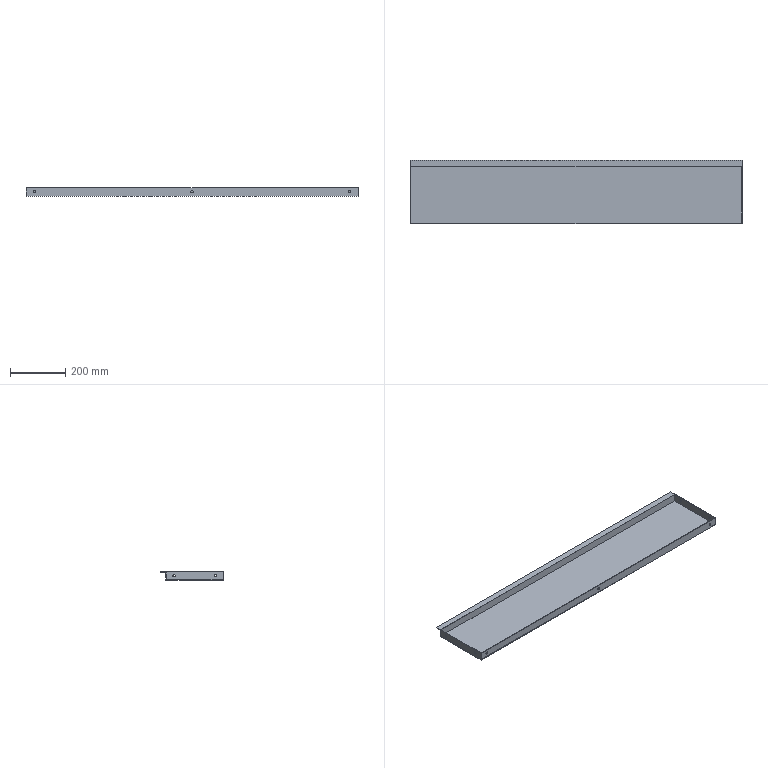Part | SolidWorks | features ICE 3, Extrusion 1, Shell 1 | 1 solid | 27 faces | box 1204 x 230 x 30 mm | volume 710869 mm3 | cylinder 14 | plane 13 | commonest cylinder face diameters 9 x14
STEP:
#1=CARTESIAN_POINT('',(602.,0.,11.5));
#2=VERTEX_POINT('',#1);
#3=CARTESIAN_POINT('',(602.,0.,20.5));
#4=VERTEX_POINT('',#3);
#5=CARTESIAN_POINT('',(602.,0.,16.));
#6=DIRECTION('',(0.,1.,0.));
#7=DIRECTION('',(0.,0.,1.));
#8=AXIS2_PLACEMENT_3D('',#5,#6,#7);
#9=CIRCLE('',#8,4.5);
#10=EDGE_CURVE('',#2,#4,#9,.T.);
#11=ORIENTED_EDGE('',*,*,#10,.F.);
#12=CARTESIAN_POINT('',(602.,2.,11.5));
#13=VERTEX_POINT('',#12);
#14=CARTESIAN_POINT('',(602.,-114.,11.5));
#15=DIRECTION('',(0.,1.,0.));
#16=VECTOR('',#15,1000.);
#17=LINE('',#14,#16);
#18=EDGE_CURVE('',#2,#13,#17,.T.);
#19=ORIENTED_EDGE('',*,*,#18,.T.);
#20=CARTESIAN_POINT('',(602.,2.,20.5));
#21=VERTEX_POINT('',#20);
#22=CARTESIAN_POINT('',(602.,2.,16.));
#23=DIRECTION('',(0.,1.,0.));
#24=DIRECTION('',(0.,0.,1.));
#25=AXIS2_PLACEMENT_3D('',#22,#23,#24);
#26=CIRCLE('',#25,4.5);
#27=EDGE_CURVE('',#13,#21,#26,.T.);
#28=ORIENTED_EDGE('',*,*,#27,.T.);
#29=CARTESIAN_POINT('',(602.,-114.,20.5));
#30=DIRECTION('',(0.,1.,0.));
#31=VECTOR('',#30,1000.);
#32=LINE('',#29,#31);
#33=EDGE_CURVE('',#4,#21,#32,.T.);
#34=ORIENTED_EDGE('',*,*,#33,.F.);
#35=EDGE_LOOP('',(#11,#19,#28,#34));
#36=FACE_OUTER_BOUND('',#35,.T.);
#37=CARTESIAN_POINT('',(602.,-114.,16.));
#38=DIRECTION('',(0.,1.,0.));
#39=DIRECTION('',(0.,0.,1.));
#40=AXIS2_PLACEMENT_3D('',#37,#38,#39);
#41=CYLINDRICAL_SURFACE('',#40,4.5);
#42=ADVANCED_FACE('',(#36),#41,.F.);
#43=CARTESIAN_POINT('',(1174.,0.,11.5));
#44=VERTEX_POINT('',#43);
#45=CARTESIAN_POINT('',(1174.,0.,20.5));
#46=VERTEX_POINT('',#45);
#47=CARTESIAN_POINT('',(1174.,0.,16.));
#48=DIRECTION('',(0.,1.,0.));
#49=DIRECTION('',(0.,0.,1.));
#50=AXIS2_PLACEMENT_3D('',#47,#48,#49);
#51=CIRCLE('',#50,4.5);
#52=EDGE_CURVE('',#44,#46,#51,.T.);
#53=ORIENTED_EDGE('',*,*,#52,.F.);
#54=CARTESIAN_POINT('',(1174.,2.,11.5));
#55=VERTEX_POINT('',#54);
#56=CARTESIAN_POINT('',(1174.,-114.,11.5));
#57=DIRECTION('',(0.,1.,0.));
#58=VECTOR('',#57,1000.);
#59=LINE('',#56,#58);
#60=EDGE_CURVE('',#44,#55,#59,.T.);
#61=ORIENTED_EDGE('',*,*,#60,.T.);
#62=CARTESIAN_POINT('',(1174.,2.,20.5));
#63=VERTEX_POINT('',#62);
#64=CARTESIAN_POINT('',(1174.,2.,16.));
#65=DIRECTION('',(0.,1.,0.));
#66=DIRECTION('',(0.,0.,1.));
#67=AXIS2_PLACEMENT_3D('',#64,#65,#66);
#68=CIRCLE('',#67,4.5);
#69=EDGE_CURVE('',#55,#63,#68,.T.);
#70=ORIENTED_EDGE('',*,*,#69,.T.);
#71=CARTESIAN_POINT('',(1174.,-114.,20.5));
#72=DIRECTION('',(0.,1.,0.));
#73=VECTOR('',#72,1000.);
#74=LINE('',#71,#73);
#75=EDGE_CURVE('',#46,#63,#74,.T.);
#76=ORIENTED_EDGE('',*,*,#75,.F.);
#77=EDGE_LOOP('',(#53,#61,#70,#76));
#78=FACE_OUTER_BOUND('',#77,.T.);
#79=CARTESIAN_POINT('',(1174.,-114.,16.));
#80=DIRECTION('',(0.,1.,0.));
#81=DIRECTION('',(0.,0.,1.));
#82=AXIS2_PLACEMENT_3D('',#79,#80,#81);
#83=CYLINDRICAL_SURFACE('',#82,4.5);
#84=ADVANCED_FACE('',(#78),#83,.F.);
#85=CARTESIAN_POINT('',(30.,0.,11.5));
#86=VERTEX_POINT('',#85);
#87=CARTESIAN_POINT('',(30.,0.,20.5));
#88=VERTEX_POINT('',#87);
#89=CARTESIAN_POINT('',(30.,0.,16.));
#90=DIRECTION('',(0.,1.,0.));
#91=DIRECTION('',(0.,0.,1.));
#92=AXIS2_PLACEMENT_3D('',#89,#90,#91);
#93=CIRCLE('',#92,4.5);
#94=EDGE_CURVE('',#86,#88,#93,.T.);
#95=ORIENTED_EDGE('',*,*,#94,.F.);
#96=CARTESIAN_POINT('',(30.,2.,11.5));
#97=VERTEX_POINT('',#96);
#98=CARTESIAN_POINT('',(30.,-114.,11.5));
#99=DIRECTION('',(0.,1.,0.));
#100=VECTOR('',#99,1000.);
#101=LINE('',#98,#100);
#102=EDGE_CURVE('',#86,#97,#101,.T.);
#103=ORIENTED_EDGE('',*,*,#102,.T.);
#104=CARTESIAN_POINT('',(30.,2.,20.5));
#105=VERTEX_POINT('',#104);
#106=CARTESIAN_POINT('',(30.,2.,16.));
#107=DIRECTION('',(0.,1.,0.));
#108=DIRECTION('',(0.,0.,1.));
#109=AXIS2_PLACEMENT_3D('',#106,#107,#108);
#110=CIRCLE('',#109,4.5);
#111=EDGE_CURVE('',#97,#105,#110,.T.);
#112=ORIENTED_EDGE('',*,*,#111,.T.);
#113=CARTESIAN_POINT('',(30.,-114.,20.5));
#114=DIRECTION('',(0.,1.,0.));
#115=VECTOR('',#114,1000.);
#116=LINE('',#113,#115);
#117=EDGE_CURVE('',#88,#105,#116,.T.);
#118=ORIENTED_EDGE('',*,*,#117,.F.);
#119=EDGE_LOOP('',(#95,#103,#112,#118));
#120=FACE_OUTER_BOUND('',#119,.T.);
#121=CARTESIAN_POINT('',(30.,-114.,16.));
#122=DIRECTION('',(0.,1.,0.));
#123=DIRECTION('',(0.,0.,1.));
#124=AXIS2_PLACEMENT_3D('',#121,#122,#123);
#125=CYLINDRICAL_SURFACE('',#124,4.5);
#126=ADVANCED_FACE('',(#120),#125,.F.);
#127=CARTESIAN_POINT('',(2.,30.,11.5));
#128=VERTEX_POINT('',#127);
#129=CARTESIAN_POINT('',(2.,30.,20.5));
#130=VERTEX_POINT('',#129);
#131=CARTESIAN_POINT('',(2.,30.,16.));
#132=DIRECTION('',(-1.,0.,0.));
#133=DIRECTION('',(0.,0.,-1.));
#134=AXIS2_PLACEMENT_3D('',#131,#132,#133);
#135=CIRCLE('',#134,4.5);
#136=EDGE_CURVE('',#128,#130,#135,.T.);
#137=ORIENTED_EDGE('',*,*,#136,.F.);
#138=CARTESIAN_POINT('',(0.,30.,11.5));
#139=VERTEX_POINT('',#138);
#140=CARTESIAN_POINT('',(1479.,30.,11.5));
#141=DIRECTION('',(-1.,0.,0.));
#142=VECTOR('',#141,1000.);
#143=LINE('',#140,#142);
#144=EDGE_CURVE('',#128,#139,#143,.T.);
#145=ORIENTED_EDGE('',*,*,#144,.T.);
#146=CARTESIAN_POINT('',(0.,30.,20.5));
#147=VERTEX_POINT('',#146);
#148=CARTESIAN_POINT('',(0.,30.,16.));
#149=DIRECTION('',(-1.,0.,0.));
#150=DIRECTION('',(0.,0.,-1.));
#151=AXIS2_PLACEMENT_3D('',#148,#149,#150);
#152=CIRCLE('',#151,4.5);
#153=EDGE_CURVE('',#139,#147,#152,.T.);
#154=ORIENTED_EDGE('',*,*,#153,.T.);
#155=CARTESIAN_POINT('',(1479.,30.,20.5));
#156=DIRECTION('',(-1.,0.,0.));
#157=VECTOR('',#156,1000.);
#158=LINE('',#155,#157);
#159=EDGE_CURVE('',#130,#147,#158,.T.);
#160=ORIENTED_EDGE('',*,*,#159,.F.);
#161=EDGE_LOOP('',(#137,#145,#154,#160));
#162=FACE_OUTER_BOUND('',#161,.T.);
#163=CARTESIAN_POINT('',(1479.,30.,16.));
#164=DIRECTION('',(-1.,0.,0.));
#165=DIRECTION('',(0.,0.,1.));
#166=AXIS2_PLACEMENT_3D('',#163,#164,#165);
#167=CYLINDRICAL_SURFACE('',#166,4.5);
#168=ADVANCED_FACE('',(#162),#167,.F.);
#169=CARTESIAN_POINT('',(1204.,30.,20.5));
#170=VERTEX_POINT('',#169);
#171=CARTESIAN_POINT('',(1204.,30.,11.5));
#172=VERTEX_POINT('',#171);
#173=CARTESIAN_POINT('',(1204.,30.,16.));
#174=DIRECTION('',(1.,0.,0.));
#175=DIRECTION('',(0.,0.,1.));
#176=AXIS2_PLACEMENT_3D('',#173,#174,#175);
#177=CIRCLE('',#176,4.5);
#178=EDGE_CURVE('',#170,#172,#177,.T.);
#179=ORIENTED_EDGE('',*,*,#178,.T.);
#180=CARTESIAN_POINT('',(1202.,30.,11.5));
#181=VERTEX_POINT('',#180);
#182=CARTESIAN_POINT('',(1479.,30.,11.5));
#183=DIRECTION('',(-1.,0.,0.));
#184=VECTOR('',#183,1000.);
#185=LINE('',#182,#184);
#186=EDGE_CURVE('',#172,#181,#185,.T.);
#187=ORIENTED_EDGE('',*,*,#186,.T.);
#188=CARTESIAN_POINT('',(1202.,30.,20.5));
#189=VERTEX_POINT('',#188);
#190=CARTESIAN_POINT('',(1202.,30.,16.));
#191=DIRECTION('',(1.,0.,0.));
#192=DIRECTION('',(0.,0.,1.));
#193=AXIS2_PLACEMENT_3D('',#190,#191,#192);
#194=CIRCLE('',#193,4.5);
#195=EDGE_CURVE('',#189,#181,#194,.T.);
#196=ORIENTED_EDGE('',*,*,#195,.F.);
#197=CARTESIAN_POINT('',(1479.,30.,20.5));
#198=DIRECTION('',(-1.,0.,0.));
#199=VECTOR('',#198,1000.);
#200=LINE('',#197,#199);
#201=EDGE_CURVE('',#170,#189,#200,.T.);
#202=ORIENTED_EDGE('',*,*,#201,.F.);
#203=EDGE_LOOP('',(#179,#187,#196,#202));
#204=FACE_OUTER_BOUND('',#203,.T.);
#205=CARTESIAN_POINT('',(1479.,30.,16.));
#206=DIRECTION('',(-1.,0.,0.));
#207=DIRECTION('',(0.,0.,1.));
#208=AXIS2_PLACEMENT_3D('',#205,#206,#207);
#209=CYLINDRICAL_SURFACE('',#208,4.5);
#210=ADVANCED_FACE('',(#204),#209,.F.);
#211=CARTESIAN_POINT('',(2.,180.,11.5));
#212=VERTEX_POINT('',#211);
#213=CARTESIAN_POINT('',(2.,180.,20.5));
#214=VERTEX_POINT('',#213);
#215=CARTESIAN_POINT('',(2.,180.,16.));
#216=DIRECTION('',(-1.,0.,0.));
#217=DIRECTION('',(0.,0.,-1.));
#218=AXIS2_PLACEMENT_3D('',#215,#216,#217);
#219=CIRCLE('',#218,4.5);
#220=EDGE_CURVE('',#212,#214,#219,.T.);
#221=ORIENTED_EDGE('',*,*,#220,.F.);
#222=CARTESIAN_POINT('',(0.,180.,11.5));
#223=VERTEX_POINT('',#222);
#224=CARTESIAN_POINT('',(1479.,180.,11.5));
#225=DIRECTION('',(-1.,0.,0.));
#226=VECTOR('',#225,1000.);
#227=LINE('',#224,#226);
#228=EDGE_CURVE('',#212,#223,#227,.T.);
#229=ORIENTED_EDGE('',*,*,#228,.T.);
#230=CARTESIAN_POINT('',(0.,180.,20.5));
#231=VERTEX_POINT('',#230);
#232=CARTESIAN_POINT('',(0.,180.,16.));
#233=DIRECTION('',(-1.,0.,0.));
#234=DIRECTION('',(0.,0.,-1.));
#235=AXIS2_PLACEMENT_3D('',#232,#233,#234);
#236=CIRCLE('',#235,4.5);
#237=EDGE_CURVE('',#223,#231,#236,.T.);
#238=ORIENTED_EDGE('',*,*,#237,.T.);
#239=CARTESIAN_POINT('',(1479.,180.,20.5));
#240=DIRECTION('',(-1.,0.,0.));
#241=VECTOR('',#240,1000.);
#242=LINE('',#239,#241);
#243=EDGE_CURVE('',#214,#231,#242,.T.);
#244=ORIENTED_EDGE('',*,*,#243,.F.);
#245=EDGE_LOOP('',(#221,#229,#238,#244));
#246=FACE_OUTER_BOUND('',#245,.T.);
#247=CARTESIAN_POINT('',(1479.,180.,16.));
#248=DIRECTION('',(-1.,0.,0.));
#249=DIRECTION('',(0.,0.,1.));
#250=AXIS2_PLACEMENT_3D('',#247,#248,#249);
#251=CYLINDRICAL_SURFACE('',#250,4.5);
#252=ADVANCED_FACE('',(#246),#251,.F.);
#253=CARTESIAN_POINT('',(1204.,180.,20.5));
#254=VERTEX_POINT('',#253);
#255=CARTESIAN_POINT('',(1204.,180.,11.5));
#256=VERTEX_POINT('',#255);
#257=CARTESIAN_POINT('',(1204.,180.,16.));
#258=DIRECTION('',(1.,0.,0.));
#259=DIRECTION('',(0.,0.,1.));
#260=AXIS2_PLACEMENT_3D('',#257,#258,#259);
#261=CIRCLE('',#260,4.5);
#262=EDGE_CURVE('',#254,#256,#261,.T.);
#263=ORIENTED_EDGE('',*,*,#262,.T.);
#264=CARTESIAN_POINT('',(1202.,180.,11.5));
#265=VERTEX_POINT('',#264);
#266=CARTESIAN_POINT('',(1479.,180.,11.5));
#267=DIRECTION('',(-1.,0.,0.));
#268=VECTOR('',#267,1000.);
#269=LINE('',#266,#268);
#270=EDGE_CURVE('',#256,#265,#269,.T.);
#271=ORIENTED_EDGE('',*,*,#270,.T.);
#272=CARTESIAN_POINT('',(1202.,180.,20.5));
#273=VERTEX_POINT('',#272);
#274=CARTESIAN_POINT('',(1202.,180.,16.));
#275=DIRECTION('',(1.,0.,0.));
#276=DIRECTION('',(0.,0.,1.));
#277=AXIS2_PLACEMENT_3D('',#274,#275,#276);
#278=CIRCLE('',#277,4.5);
#279=EDGE_CURVE('',#273,#265,#278,.T.);
#280=ORIENTED_EDGE('',*,*,#279,.F.);
#281=CARTESIAN_POINT('',(1479.,180.,20.5));
#282=DIRECTION('',(-1.,0.,0.));
#283=VECTOR('',#282,1000.);
#284=LINE('',#281,#283);
#285=EDGE_CURVE('',#254,#273,#284,.T.);
#286=ORIENTED_EDGE('',*,*,#285,.F.);
#287=EDGE_LOOP('',(#263,#271,#280,#286));
#288=FACE_OUTER_BOUND('',#287,.T.);
#289=CARTESIAN_POINT('',(1479.,180.,16.));
#290=DIRECTION('',(-1.,0.,0.));
#291=DIRECTION('',(0.,0.,1.));
#292=AXIS2_PLACEMENT_3D('',#289,#290,#291);
#293=CYLINDRICAL_SURFACE('',#292,4.5);
#294=ADVANCED_FACE('',(#288),#293,.F.);
#295=CARTESIAN_POINT('',(0.,180.,16.));
#296=DIRECTION('',(-1.,0.,0.));
#297=DIRECTION('',(0.,0.,-1.));
#298=AXIS2_PLACEMENT_3D('',#295,#296,#297);
#299=CIRCLE('',#298,4.5);
#300=EDGE_CURVE('',#231,#223,#299,.T.);
#301=ORIENTED_EDGE('',*,*,#300,.F.);
#302=ORIENTED_EDGE('',*,*,#237,.F.);
#303=EDGE_LOOP('',(#301,#302));
#304=FACE_BOUND('',#303,.T.);
#305=CARTESIAN_POINT('',(0.,210.,0.));
#306=VERTEX_POINT('',#305);
#307=CARTESIAN_POINT('',(0.,0.,0.));
#308=VERTEX_POINT('',#307);
#309=CARTESIAN_POINT('',(0.,0.,0.));
#310=DIRECTION('',(0.,-1.,0.));
#311=VECTOR('',#310,1000.);
#312=LINE('',#309,#311);
#313=EDGE_CURVE('',#306,#308,#312,.T.);
#314=ORIENTED_EDGE('',*,*,#313,.T.);
#315=CARTESIAN_POINT('',(0.,0.,30.));
#316=VERTEX_POINT('',#315);
#317=CARTESIAN_POINT('',(0.,0.,30.));
#318=DIRECTION('',(0.,0.,-1.));
#319=VECTOR('',#318,1000.);
#320=LINE('',#317,#319);
#321=EDGE_CURVE('',#316,#308,#320,.T.);
#322=ORIENTED_EDGE('',*,*,#321,.F.);
#323=CARTESIAN_POINT('',(0.,230.,30.));
#324=VERTEX_POINT('',#323);
#325=CARTESIAN_POINT('',(0.,0.,30.));
#326=DIRECTION('',(0.,-1.,0.));
#327=VECTOR('',#326,1000.);
#328=LINE('',#325,#327);
#329=EDGE_CURVE('',#324,#316,#328,.T.);
#330=ORIENTED_EDGE('',*,*,#329,.F.);
#331=CARTESIAN_POINT('',(0.,230.,28.));
#332=VERTEX_POINT('',#331);
#333=CARTESIAN_POINT('',(0.,230.,28.));
#334=DIRECTION('',(0.,0.,1.));
#335=VECTOR('',#334,1000.);
#336=LINE('',#333,#335);
#337=EDGE_CURVE('',#332,#324,#336,.T.);
#338=ORIENTED_EDGE('',*,*,#337,.F.);
#339=CARTESIAN_POINT('',(0.,210.,28.));
#340=VERTEX_POINT('',#339);
#341=CARTESIAN_POINT('',(0.,230.,28.));
#342=DIRECTION('',(0.,-1.,0.));
#343=VECTOR('',#342,1000.);
#344=LINE('',#341,#343);
#345=EDGE_CURVE('',#332,#340,#344,.T.);
#346=ORIENTED_EDGE('',*,*,#345,.T.);
#347=CARTESIAN_POINT('',(0.,210.,30.));
#348=DIRECTION('',(0.,0.,-1.));
#349=VECTOR('',#348,1000.);
#350=LINE('',#347,#349);
#351=EDGE_CURVE('',#340,#306,#350,.T.);
#352=ORIENTED_EDGE('',*,*,#351,.T.);
#353=EDGE_LOOP('',(#314,#322,#330,#338,#346,#352));
#354=FACE_OUTER_BOUND('',#353,.T.);
#355=CARTESIAN_POINT('',(0.,30.,16.));
#356=DIRECTION('',(-1.,0.,0.));
#357=DIRECTION('',(0.,0.,-1.));
#358=AXIS2_PLACEMENT_3D('',#355,#356,#357);
#359=CIRCLE('',#358,4.5);
#360=EDGE_CURVE('',#147,#139,#359,.T.);
#361=ORIENTED_EDGE('',*,*,#360,.F.);
#362=ORIENTED_EDGE('',*,*,#153,.F.);
#363=EDGE_LOOP('',(#361,#362));
#364=FACE_BOUND('',#363,.T.);
#365=CARTESIAN_POINT('',(0.,0.,30.));
#366=DIRECTION('',(1.,0.,0.));
#367=DIRECTION('',(0.,0.,-1.));
#368=AXIS2_PLACEMENT_3D('',#365,#366,#367);
#369=PLANE('',#368);
#370=ADVANCED_FACE('',(#304,#354,#364),#369,.F.);
#371=ORIENTED_EDGE('',*,*,#262,.F.);
#372=CARTESIAN_POINT('',(1204.,180.,16.));
#373=DIRECTION('',(1.,0.,0.));
#374=DIRECTION('',(0.,0.,1.));
#375=AXIS2_PLACEMENT_3D('',#372,#373,#374);
#376=CIRCLE('',#375,4.5);
#377=EDGE_CURVE('',#256,#254,#376,.T.);
#378=ORIENTED_EDGE('',*,*,#377,.F.);
#379=EDGE_LOOP('',(#371,#378));
#380=FACE_BOUND('',#379,.T.);
#381=CARTESIAN_POINT('',(1204.,0.,0.));
#382=VERTEX_POINT('',#381);
#383=CARTESIAN_POINT('',(1204.,210.,0.));
#384=VERTEX_POINT('',#383);
#385=CARTESIAN_POINT('',(1204.,0.,0.));
#386=DIRECTION('',(0.,1.,0.));
#387=VECTOR('',#386,1000.);
#388=LINE('',#385,#387);
#389=EDGE_CURVE('',#382,#384,#388,.T.);
#390=ORIENTED_EDGE('',*,*,#389,.T.);
#391=CARTESIAN_POINT('',(1204.,210.,28.));
#392=VERTEX_POINT('',#391);
#393=CARTESIAN_POINT('',(1204.,210.,30.));
#394=DIRECTION('',(0.,0.,-1.));
#395=VECTOR('',#394,1000.);
#396=LINE('',#393,#395);
#397=EDGE_CURVE('',#392,#384,#396,.T.);
#398=ORIENTED_EDGE('',*,*,#397,.F.);
#399=CARTESIAN_POINT('',(1204.,230.,28.));
#400=VERTEX_POINT('',#399);
#401=CARTESIAN_POINT('',(1204.,210.,28.));
#402=DIRECTION('',(0.,1.,0.));
#403=VECTOR('',#402,1000.);
#404=LINE('',#401,#403);
#405=EDGE_CURVE('',#392,#400,#404,.T.);
#406=ORIENTED_EDGE('',*,*,#405,.T.);
#407=CARTESIAN_POINT('',(1204.,230.,30.));
#408=VERTEX_POINT('',#407);
#409=CARTESIAN_POINT('',(1204.,230.,28.));
#410=DIRECTION('',(0.,0.,1.));
#411=VECTOR('',#410,1000.);
#412=LINE('',#409,#411);
#413=EDGE_CURVE('',#400,#408,#412,.T.);
#414=ORIENTED_EDGE('',*,*,#413,.T.);
#415=CARTESIAN_POINT('',(1204.,0.,30.));
#416=VERTEX_POINT('',#415);
#417=CARTESIAN_POINT('',(1204.,0.,30.));
#418=DIRECTION('',(0.,1.,0.));
#419=VECTOR('',#418,1000.);
#420=LINE('',#417,#419);
#421=EDGE_CURVE('',#416,#408,#420,.T.);
#422=ORIENTED_EDGE('',*,*,#421,.F.);
#423=CARTESIAN_POINT('',(1204.,0.,30.));
#424=DIRECTION('',(0.,0.,-1.));
#425=VECTOR('',#424,1000.);
#426=LINE('',#423,#425);
#427=EDGE_CURVE('',#416,#382,#426,.T.);
#428=ORIENTED_EDGE('',*,*,#427,.T.);
#429=EDGE_LOOP('',(#390,#398,#406,#414,#422,#428));
#430=FACE_OUTER_BOUND('',#429,.T.);
#431=ORIENTED_EDGE('',*,*,#178,.F.);
#432=CARTESIAN_POINT('',(1204.,30.,16.));
#433=DIRECTION('',(1.,0.,0.));
#434=DIRECTION('',(0.,0.,1.));
#435=AXIS2_PLACEMENT_3D('',#432,#433,#434);
#436=CIRCLE('',#435,4.5);
#437=EDGE_CURVE('',#172,#170,#436,.T.);
#438=ORIENTED_EDGE('',*,*,#437,.F.);
#439=EDGE_LOOP('',(#431,#438));
#440=FACE_BOUND('',#439,.T.);
#441=CARTESIAN_POINT('',(1204.,0.,30.));
#442=DIRECTION('',(-1.,0.,0.));
#443=DIRECTION('',(0.,0.,1.));
#444=AXIS2_PLACEMENT_3D('',#441,#442,#443);
#445=PLANE('',#444);
#446=ADVANCED_FACE('',(#380,#430,#440),#445,.F.);
#447=CARTESIAN_POINT('',(2.,180.,16.));
#448=DIRECTION('',(-1.,0.,0.));
#449=DIRECTION('',(0.,0.,-1.));
#450=AXIS2_PLACEMENT_3D('',#447,#448,#449);
#451=CIRCLE('',#450,4.5);
#452=EDGE_CURVE('',#214,#212,#451,.T.);
#453=ORIENTED_EDGE('',*,*,#452,.T.);
#454=ORIENTED_EDGE('',*,*,#220,.T.);
#455=EDGE_LOOP('',(#453,#454));
#456=FACE_BOUND('',#455,.T.);
#457=CARTESIAN_POINT('',(2.,208.,2.));
#458=VERTEX_POINT('',#457);
#459=CARTESIAN_POINT('',(2.,2.,2.));
#460=VERTEX_POINT('',#459);
#461=CARTESIAN_POINT('',(2.,210.,2.));
#462=DIRECTION('',(0.,-1.,0.));
#463=VECTOR('',#462,1000.);
#464=LINE('',#461,#463);
#465=EDGE_CURVE('',#458,#460,#464,.T.);
#466=ORIENTED_EDGE('',*,*,#465,.F.);
#467=CARTESIAN_POINT('',(2.,208.,30.));
#468=VERTEX_POINT('',#467);
#469=CARTESIAN_POINT('',(2.,208.,30.));
#470=DIRECTION('',(0.,0.,-1.));
#471=VECTOR('',#470,1000.);
#472=LINE('',#469,#471);
#473=EDGE_CURVE('',#468,#458,#472,.T.);
#474=ORIENTED_EDGE('',*,*,#473,.F.);
#475=CARTESIAN_POINT('',(2.,2.,30.));
#476=VERTEX_POINT('',#475);
#477=CARTESIAN_POINT('',(2.,210.,30.));
#478=DIRECTION('',(0.,-1.,0.));
#479=VECTOR('',#478,1000.);
#480=LINE('',#477,#479);
#481=EDGE_CURVE('',#468,#476,#480,.T.);
#482=ORIENTED_EDGE('',*,*,#481,.T.);
#483=CARTESIAN_POINT('',(2.,2.,30.));
#484=DIRECTION('',(0.,0.,-1.));
#485=VECTOR('',#484,1000.);
#486=LINE('',#483,#485);
#487=EDGE_CURVE('',#476,#460,#486,.T.);
#488=ORIENTED_EDGE('',*,*,#487,.T.);
#489=EDGE_LOOP('',(#466,#474,#482,#488));
#490=FACE_OUTER_BOUND('',#489,.T.);
#491=CARTESIAN_POINT('',(2.,30.,16.));
#492=DIRECTION('',(-1.,0.,0.));
#493=DIRECTION('',(0.,0.,-1.));
#494=AXIS2_PLACEMENT_3D('',#491,#492,#493);
#495=CIRCLE('',#494,4.5);
#496=EDGE_CURVE('',#130,#128,#495,.T.);
#497=ORIENTED_EDGE('',*,*,#496,.T.);
#498=ORIENTED_EDGE('',*,*,#136,.T.);
#499=EDGE_LOOP('',(#497,#498));
#500=FACE_BOUND('',#499,.T.);
#501=CARTESIAN_POINT('',(2.,0.,30.));
#502=DIRECTION('',(1.,0.,0.));
#503=DIRECTION('',(0.,0.,-1.));
#504=AXIS2_PLACEMENT_3D('',#501,#502,#503);
#505=PLANE('',#504);
#506=ADVANCED_FACE('',(#456,#490,#500),#505,.T.);
#507=ORIENTED_EDGE('',*,*,#279,.T.);
#508=CARTESIAN_POINT('',(1202.,180.,16.));
#509=DIRECTION('',(1.,0.,0.));
#510=DIRECTION('',(0.,0.,1.));
#511=AXIS2_PLACEMENT_3D('',#508,#509,#510);
#512=CIRCLE('',#511,4.5);
#513=EDGE_CURVE('',#265,#273,#512,.T.);
#514=ORIENTED_EDGE('',*,*,#513,.T.);
#515=EDGE_LOOP('',(#507,#514));
#516=FACE_BOUND('',#515,.T.);
#517=CARTESIAN_POINT('',(1202.,2.,2.));
#518=VERTEX_POINT('',#517);
#519=CARTESIAN_POINT('',(1202.,208.,2.));
#520=VERTEX_POINT('',#519);
#521=CARTESIAN_POINT('',(1202.,210.,2.));
#522=DIRECTION('',(0.,1.,0.));
#523=VECTOR('',#522,1000.);
#524=LINE('',#521,#523);
#525=EDGE_CURVE('',#518,#520,#524,.T.);
#526=ORIENTED_EDGE('',*,*,#525,.F.);
#527=CARTESIAN_POINT('',(1202.,2.,30.));
#528=VERTEX_POINT('',#527);
#529=CARTESIAN_POINT('',(1202.,2.,30.));
#530=DIRECTION('',(0.,0.,-1.));
#531=VECTOR('',#530,1000.);
#532=LINE('',#529,#531);
#533=EDGE_CURVE('',#528,#518,#532,.T.);
#534=ORIENTED_EDGE('',*,*,#533,.F.);
#535=CARTESIAN_POINT('',(1202.,208.,30.));
#536=VERTEX_POINT('',#535);
#537=CARTESIAN_POINT('',(1202.,210.,30.));
#538=DIRECTION('',(0.,1.,0.));
#539=VECTOR('',#538,1000.);
#540=LINE('',#537,#539);
#541=EDGE_CURVE('',#528,#536,#540,.T.);
#542=ORIENTED_EDGE('',*,*,#541,.T.);
#543=CARTESIAN_POINT('',(1202.,208.,30.));
#544=DIRECTION('',(0.,0.,-1.));
#545=VECTOR('',#544,1000.);
#546=LINE('',#543,#545);
#547=EDGE_CURVE('',#536,#520,#546,.T.);
#548=ORIENTED_EDGE('',*,*,#547,.T.);
#549=EDGE_LOOP('',(#526,#534,#542,#548));
#550=FACE_OUTER_BOUND('',#549,.T.);
#551=ORIENTED_EDGE('',*,*,#195,.T.);
#552=CARTESIAN_POINT('',(1202.,30.,16.));
#553=DIRECTION('',(1.,0.,0.));
#554=DIRECTION('',(0.,0.,1.));
#555=AXIS2_PLACEMENT_3D('',#552,#553,#554);
#556=CIRCLE('',#555,4.5);
#557=EDGE_CURVE('',#181,#189,#556,.T.);
#558=ORIENTED_EDGE('',*,*,#557,.T.);
#559=EDGE_LOOP('',(#551,#558));
#560=FACE_BOUND('',#559,.T.);
#561=CARTESIAN_POINT('',(1202.,0.,30.));
#562=DIRECTION('',(-1.,0.,0.));
#563=DIRECTION('',(0.,0.,1.));
#564=AXIS2_PLACEMENT_3D('',#561,#562,#563);
#565=PLANE('',#564);
#566=ADVANCED_FACE('',(#516,#550,#560),#565,.T.);
#567=ORIENTED_EDGE('',*,*,#329,.T.);
#568=CARTESIAN_POINT('',(0.,0.,30.));
#569=DIRECTION('',(1.,0.,0.));
#570=VECTOR('',#569,1000.);
#571=LINE('',#568,#570);
#572=EDGE_CURVE('',#316,#416,#571,.T.);
#573=ORIENTED_EDGE('',*,*,#572,.T.);
#574=ORIENTED_EDGE('',*,*,#421,.T.);
#575=CARTESIAN_POINT('',(0.,230.,30.));
#576=DIRECTION('',(-1.,0.,0.));
#577=VECTOR('',#576,1000.);
#578=LINE('',#575,#577);
#579=EDGE_CURVE('',#408,#324,#578,.T.);
#580=ORIENTED_EDGE('',*,*,#579,.T.);
#581=EDGE_LOOP('',(#567,#573,#574,#580));
#582=FACE_OUTER_BOUND('',#581,.T.);
#583=ORIENTED_EDGE('',*,*,#481,.F.);
#584=CARTESIAN_POINT('',(0.,208.,30.));
#585=DIRECTION('',(-1.,0.,0.));
#586=VECTOR('',#585,1000.);
#587=LINE('',#584,#586);
#588=EDGE_CURVE('',#536,#468,#587,.T.);
#589=ORIENTED_EDGE('',*,*,#588,.F.);
#590=ORIENTED_EDGE('',*,*,#541,.F.);
#591=CARTESIAN_POINT('',(0.,2.,30.));
#592=DIRECTION('',(1.,0.,0.));
#593=VECTOR('',#592,1000.);
#594=LINE('',#591,#593);
#595=EDGE_CURVE('',#476,#528,#594,.T.);
#596=ORIENTED_EDGE('',*,*,#595,.F.);
#597=EDGE_LOOP('',(#583,#589,#590,#596));
#598=FACE_BOUND('',#597,.T.);
#599=CARTESIAN_POINT('',(0.,210.,30.));
#600=DIRECTION('',(0.,0.,-1.));
#601=DIRECTION('',(-1.,0.,0.));
#602=AXIS2_PLACEMENT_3D('',#599,#600,#601);
#603=PLANE('',#602);
#604=ADVANCED_FACE('',(#582,#598),#603,.F.);
#605=CARTESIAN_POINT('',(602.,0.,16.));
#606=DIRECTION('',(0.,1.,0.));
#607=DIRECTION('',(0.,0.,1.));
#608=AXIS2_PLACEMENT_3D('',#605,#606,#607);
#609=CIRCLE('',#608,4.5);
#610=EDGE_CURVE('',#4,#2,#609,.T.);
#611=ORIENTED_EDGE('',*,*,#610,.T.);
#612=ORIENTED_EDGE('',*,*,#10,.T.);
#613=EDGE_LOOP('',(#611,#612));
#614=FACE_BOUND('',#613,.T.);
#615=CARTESIAN_POINT('',(1174.,0.,16.));
#616=DIRECTION('',(0.,1.,0.));
#617=DIRECTION('',(0.,0.,1.));
#618=AXIS2_PLACEMENT_3D('',#615,#616,#617);
#619=CIRCLE('',#618,4.5);
#620=EDGE_CURVE('',#46,#44,#619,.T.);
#621=ORIENTED_EDGE('',*,*,#620,.T.);
#622=ORIENTED_EDGE('',*,*,#52,.T.);
#623=EDGE_LOOP('',(#621,#622));
#624=FACE_BOUND('',#623,.T.);
#625=CARTESIAN_POINT('',(30.,0.,16.));
#626=DIRECTION('',(0.,1.,0.));
#627=DIRECTION('',(0.,0.,1.));
#628=AXIS2_PLACEMENT_3D('',#625,#626,#627);
#629=CIRCLE('',#628,4.5);
#630=EDGE_CURVE('',#88,#86,#629,.T.);
#631=ORIENTED_EDGE('',*,*,#630,.T.);
#632=ORIENTED_EDGE('',*,*,#94,.T.);
#633=EDGE_LOOP('',(#631,#632));
#634=FACE_BOUND('',#633,.T.);
#635=CARTESIAN_POINT('',(0.,0.,0.));
#636=DIRECTION('',(1.,0.,0.));
#637=VECTOR('',#636,1000.);
#638=LINE('',#635,#637);
#639=EDGE_CURVE('',#308,#382,#638,.T.);
#640=ORIENTED_EDGE('',*,*,#639,.T.);
#641=ORIENTED_EDGE('',*,*,#427,.F.);
#642=ORIENTED_EDGE('',*,*,#572,.F.);
#643=ORIENTED_EDGE('',*,*,#321,.T.);
#644=EDGE_LOOP('',(#640,#641,#642,#643));
#645=FACE_OUTER_BOUND('',#644,.T.);
#646=CARTESIAN_POINT('',(0.,0.,30.));
#647=DIRECTION('',(0.,1.,0.));
#648=DIRECTION('',(0.,0.,1.));
#649=AXIS2_PLACEMENT_3D('',#646,#647,#648);
#650=PLANE('',#649);
#651=ADVANCED_FACE('',(#614,#624,#634,#645),#650,.F.);
#652=ORIENTED_EDGE('',*,*,#351,.F.);
#653=CARTESIAN_POINT('',(0.,210.,28.));
#654=DIRECTION('',(1.,0.,0.));
#655=VECTOR('',#654,1000.);
#656=LINE('',#653,#655);
#657=EDGE_CURVE('',#340,#392,#656,.T.);
#658=ORIENTED_EDGE('',*,*,#657,.T.);
#659=ORIENTED_EDGE('',*,*,#397,.T.);
#660=CARTESIAN_POINT('',(0.,210.,0.));
#661=DIRECTION('',(-1.,0.,0.));
#662=VECTOR('',#661,1000.);
#663=LINE('',#660,#662);
#664=EDGE_CURVE('',#384,#306,#663,.T.);
#665=ORIENTED_EDGE('',*,*,#664,.T.);
#666=EDGE_LOOP('',(#652,#658,#659,#665));
#667=FACE_OUTER_BOUND('',#666,.T.);
#668=CARTESIAN_POINT('',(0.,210.,30.));
#669=DIRECTION('',(0.,-1.,0.));
#670=DIRECTION('',(0.,0.,-1.));
#671=AXIS2_PLACEMENT_3D('',#668,#669,#670);
#672=PLANE('',#671);
#673=ADVANCED_FACE('',(#667),#672,.F.);
#674=ORIENTED_EDGE('',*,*,#313,.F.);
#675=ORIENTED_EDGE('',*,*,#664,.F.);
#676=ORIENTED_EDGE('',*,*,#389,.F.);
#677=ORIENTED_EDGE('',*,*,#639,.F.);
#678=EDGE_LOOP('',(#674,#675,#676,#677));
#679=FACE_OUTER_BOUND('',#678,.T.);
#680=CARTESIAN_POINT('',(0.,210.,0.));
#681=DIRECTION('',(0.,0.,-1.));
#682=DIRECTION('',(-1.,0.,0.));
#683=AXIS2_PLACEMENT_3D('',#680,#681,#682);
#684=PLANE('',#683);
#685=ADVANCED_FACE('',(#679),#684,.T.);
#686=CARTESIAN_POINT('',(602.,2.,16.));
#687=DIRECTION('',(0.,1.,0.));
#688=DIRECTION('',(0.,0.,1.));
#689=AXIS2_PLACEMENT_3D('',#686,#687,#688);
#690=CIRCLE('',#689,4.5);
#691=EDGE_CURVE('',#21,#13,#690,.T.);
#692=ORIENTED_EDGE('',*,*,#691,.F.);
#693=ORIENTED_EDGE('',*,*,#27,.F.);
#694=EDGE_LOOP('',(#692,#693));
#695=FACE_BOUND('',#694,.T.);
#696=CARTESIAN_POINT('',(1174.,2.,16.));
#697=DIRECTION('',(0.,1.,0.));
#698=DIRECTION('',(0.,0.,1.));
#699=AXIS2_PLACEMENT_3D('',#696,#697,#698);
#700=CIRCLE('',#699,4.5);
#701=EDGE_CURVE('',#63,#55,#700,.T.);
#702=ORIENTED_EDGE('',*,*,#701,.F.);
#703=ORIENTED_EDGE('',*,*,#69,.F.);
#704=EDGE_LOOP('',(#702,#703));
#705=FACE_BOUND('',#704,.T.);
#706=CARTESIAN_POINT('',(30.,2.,16.));
#707=DIRECTION('',(0.,1.,0.));
#708=DIRECTION('',(0.,0.,1.));
#709=AXIS2_PLACEMENT_3D('',#706,#707,#708);
#710=CIRCLE('',#709,4.5);
#711=EDGE_CURVE('',#105,#97,#710,.T.);
#712=ORIENTED_EDGE('',*,*,#711,.F.);
#713=ORIENTED_EDGE('',*,*,#111,.F.);
#714=EDGE_LOOP('',(#712,#713));
#715=FACE_BOUND('',#714,.T.);
#716=CARTESIAN_POINT('',(0.,2.,2.));
#717=DIRECTION('',(1.,0.,0.));
#718=VECTOR('',#717,1000.);
#719=LINE('',#716,#718);
#720=EDGE_CURVE('',#460,#518,#719,.T.);
#721=ORIENTED_EDGE('',*,*,#720,.F.);
#722=ORIENTED_EDGE('',*,*,#487,.F.);
#723=ORIENTED_EDGE('',*,*,#595,.T.);
#724=ORIENTED_EDGE('',*,*,#533,.T.);
#725=EDGE_LOOP('',(#721,#722,#723,#724));
#726=FACE_OUTER_BOUND('',#725,.T.);
#727=CARTESIAN_POINT('',(0.,2.,30.));
#728=DIRECTION('',(0.,1.,0.));
#729=DIRECTION('',(0.,0.,1.));
#730=AXIS2_PLACEMENT_3D('',#727,#728,#729);
#731=PLANE('',#730);
#732=ADVANCED_FACE('',(#695,#705,#715,#726),#731,.T.);
#733=CARTESIAN_POINT('',(0.,208.,2.));
#734=DIRECTION('',(-1.,0.,0.));
#735=VECTOR('',#734,1000.);
#736=LINE('',#733,#735);
#737=EDGE_CURVE('',#520,#458,#736,.T.);
#738=ORIENTED_EDGE('',*,*,#737,.F.);
#739=ORIENTED_EDGE('',*,*,#547,.F.);
#740=ORIENTED_EDGE('',*,*,#588,.T.);
#741=ORIENTED_EDGE('',*,*,#473,.T.);
#742=EDGE_LOOP('',(#738,#739,#740,#741));
#743=FACE_OUTER_BOUND('',#742,.T.);
#744=CARTESIAN_POINT('',(0.,208.,30.));
#745=DIRECTION('',(0.,-1.,0.));
#746=DIRECTION('',(0.,0.,-1.));
#747=AXIS2_PLACEMENT_3D('',#744,#745,#746);
#748=PLANE('',#747);
#749=ADVANCED_FACE('',(#743),#748,.T.);
#750=ORIENTED_EDGE('',*,*,#465,.T.);
#751=ORIENTED_EDGE('',*,*,#720,.T.);
#752=ORIENTED_EDGE('',*,*,#525,.T.);
#753=ORIENTED_EDGE('',*,*,#737,.T.);
#754=EDGE_LOOP('',(#750,#751,#752,#753));
#755=FACE_OUTER_BOUND('',#754,.T.);
#756=CARTESIAN_POINT('',(0.,210.,2.));
#757=DIRECTION('',(0.,0.,-1.));
#758=DIRECTION('',(-1.,0.,0.));
#759=AXIS2_PLACEMENT_3D('',#756,#757,#758);
#760=PLANE('',#759);
#761=ADVANCED_FACE('',(#755),#760,.F.);
#762=ORIENTED_EDGE('',*,*,#579,.F.);
#763=ORIENTED_EDGE('',*,*,#413,.F.);
#764=CARTESIAN_POINT('',(0.,230.,28.));
#765=DIRECTION('',(-1.,0.,0.));
#766=VECTOR('',#765,1000.);
#767=LINE('',#764,#766);
#768=EDGE_CURVE('',#400,#332,#767,.T.);
#769=ORIENTED_EDGE('',*,*,#768,.T.);
#770=ORIENTED_EDGE('',*,*,#337,.T.);
#771=EDGE_LOOP('',(#762,#763,#769,#770));
#772=FACE_OUTER_BOUND('',#771,.T.);
#773=CARTESIAN_POINT('',(0.,230.,28.));
#774=DIRECTION('',(0.,1.,0.));
#775=DIRECTION('',(-1.,0.,0.));
#776=AXIS2_PLACEMENT_3D('',#773,#774,#775);
#777=PLANE('',#776);
#778=ADVANCED_FACE('',(#772),#777,.T.);
#779=ORIENTED_EDGE('',*,*,#345,.F.);
#780=ORIENTED_EDGE('',*,*,#768,.F.);
#781=ORIENTED_EDGE('',*,*,#405,.F.);
#782=ORIENTED_EDGE('',*,*,#657,.F.);
#783=EDGE_LOOP('',(#779,#780,#781,#782));
#784=FACE_OUTER_BOUND('',#783,.T.);
#785=CARTESIAN_POINT('',(0.,210.,28.));
#786=DIRECTION('',(0.,0.,1.));
#787=DIRECTION('',(1.,0.,0.));
#788=AXIS2_PLACEMENT_3D('',#785,#786,#787);
#789=PLANE('',#788);
#790=ADVANCED_FACE('',(#784),#789,.F.);
#791=ORIENTED_EDGE('',*,*,#270,.F.);
#792=ORIENTED_EDGE('',*,*,#377,.T.);
#793=ORIENTED_EDGE('',*,*,#285,.T.);
#794=ORIENTED_EDGE('',*,*,#513,.F.);
#795=EDGE_LOOP('',(#791,#792,#793,#794));
#796=FACE_OUTER_BOUND('',#795,.T.);
#797=CARTESIAN_POINT('',(1479.,180.,16.));
#798=DIRECTION('',(-1.,0.,0.));
#799=DIRECTION('',(0.,0.,1.));
#800=AXIS2_PLACEMENT_3D('',#797,#798,#799);
#801=CYLINDRICAL_SURFACE('',#800,4.5);
#802=ADVANCED_FACE('',(#796),#801,.F.);
#803=ORIENTED_EDGE('',*,*,#228,.F.);
#804=ORIENTED_EDGE('',*,*,#452,.F.);
#805=ORIENTED_EDGE('',*,*,#243,.T.);
#806=ORIENTED_EDGE('',*,*,#300,.T.);
#807=EDGE_LOOP('',(#803,#804,#805,#806));
#808=FACE_OUTER_BOUND('',#807,.T.);
#809=CARTESIAN_POINT('',(1479.,180.,16.));
#810=DIRECTION('',(-1.,0.,0.));
#811=DIRECTION('',(0.,0.,1.));
#812=AXIS2_PLACEMENT_3D('',#809,#810,#811);
#813=CYLINDRICAL_SURFACE('',#812,4.5);
#814=ADVANCED_FACE('',(#808),#813,.F.);
#815=ORIENTED_EDGE('',*,*,#186,.F.);
#816=ORIENTED_EDGE('',*,*,#437,.T.);
#817=ORIENTED_EDGE('',*,*,#201,.T.);
#818=ORIENTED_EDGE('',*,*,#557,.F.);
#819=EDGE_LOOP('',(#815,#816,#817,#818));
#820=FACE_OUTER_BOUND('',#819,.T.);
#821=CARTESIAN_POINT('',(1479.,30.,16.));
#822=DIRECTION('',(-1.,0.,0.));
#823=DIRECTION('',(0.,0.,1.));
#824=AXIS2_PLACEMENT_3D('',#821,#822,#823);
#825=CYLINDRICAL_SURFACE('',#824,4.5);
#826=ADVANCED_FACE('',(#820),#825,.F.);
#827=ORIENTED_EDGE('',*,*,#144,.F.);
#828=ORIENTED_EDGE('',*,*,#496,.F.);
#829=ORIENTED_EDGE('',*,*,#159,.T.);
#830=ORIENTED_EDGE('',*,*,#360,.T.);
#831=EDGE_LOOP('',(#827,#828,#829,#830));
#832=FACE_OUTER_BOUND('',#831,.T.);
#833=CARTESIAN_POINT('',(1479.,30.,16.));
#834=DIRECTION('',(-1.,0.,0.));
#835=DIRECTION('',(0.,0.,1.));
#836=AXIS2_PLACEMENT_3D('',#833,#834,#835);
#837=CYLINDRICAL_SURFACE('',#836,4.5);
#838=ADVANCED_FACE('',(#832),#837,.F.);
#839=ORIENTED_EDGE('',*,*,#102,.F.);
#840=ORIENTED_EDGE('',*,*,#630,.F.);
#841=ORIENTED_EDGE('',*,*,#117,.T.);
#842=ORIENTED_EDGE('',*,*,#711,.T.);
#843=EDGE_LOOP('',(#839,#840,#841,#842));
#844=FACE_OUTER_BOUND('',#843,.T.);
#845=CARTESIAN_POINT('',(30.,-114.,16.));
#846=DIRECTION('',(0.,1.,0.));
#847=DIRECTION('',(0.,0.,1.));
#848=AXIS2_PLACEMENT_3D('',#845,#846,#847);
#849=CYLINDRICAL_SURFACE('',#848,4.5);
#850=ADVANCED_FACE('',(#844),#849,.F.);
#851=ORIENTED_EDGE('',*,*,#60,.F.);
#852=ORIENTED_EDGE('',*,*,#620,.F.);
#853=ORIENTED_EDGE('',*,*,#75,.T.);
#854=ORIENTED_EDGE('',*,*,#701,.T.);
#855=EDGE_LOOP('',(#851,#852,#853,#854));
#856=FACE_OUTER_BOUND('',#855,.T.);
#857=CARTESIAN_POINT('',(1174.,-114.,16.));
#858=DIRECTION('',(0.,1.,0.));
#859=DIRECTION('',(0.,0.,1.));
#860=AXIS2_PLACEMENT_3D('',#857,#858,#859);
#861=CYLINDRICAL_SURFACE('',#860,4.5);
#862=ADVANCED_FACE('',(#856),#861,.F.);
#863=ORIENTED_EDGE('',*,*,#18,.F.);
#864=ORIENTED_EDGE('',*,*,#610,.F.);
#865=ORIENTED_EDGE('',*,*,#33,.T.);
#866=ORIENTED_EDGE('',*,*,#691,.T.);
#867=EDGE_LOOP('',(#863,#864,#865,#866));
#868=FACE_OUTER_BOUND('',#867,.T.);
#869=CARTESIAN_POINT('',(602.,-114.,16.));
#870=DIRECTION('',(0.,1.,0.));
#871=DIRECTION('',(0.,0.,1.));
#872=AXIS2_PLACEMENT_3D('',#869,#870,#871);
#873=CYLINDRICAL_SURFACE('',#872,4.5);
#874=ADVANCED_FACE('',(#868),#873,.F.);
#875=CLOSED_SHELL('',(#42,#84,#126,#168,#210,#252,#294,#370,#446,#506,#566,#604,#651,#673,#685,#732,#749,#761,#778,#790,#802,#814,#826,#838,#850,#862,#874));
#876=MANIFOLD_SOLID_BREP('',#875);
#877=CARTESIAN_POINT('',(0.,0.,0.));
#878=DIRECTION('',(0.,0.,1.));
#879=DIRECTION('',(1.,0.,0.));
#880=AXIS2_PLACEMENT_3D('',#877,#878,#879);
#881=(LENGTH_UNIT()NAMED_UNIT(*)SI_UNIT(.MILLI.,.METRE.));
#882=UNCERTAINTY_MEASURE_WITH_UNIT(LENGTH_MEASURE(0.00001),#881,'','');
#883=(NAMED_UNIT(*)PLANE_ANGLE_UNIT()SI_UNIT($,.RADIAN.));
#884=(NAMED_UNIT(*)SI_UNIT($,.STERADIAN.)SOLID_ANGLE_UNIT());
#885=(GEOMETRIC_REPRESENTATION_CONTEXT(3)GLOBAL_UNCERTAINTY_ASSIGNED_CONTEXT((#882))GLOBAL_UNIT_ASSIGNED_CONTEXT((#881,#883,#884))REPRESENTATION_CONTEXT('',''));
#886=ADVANCED_BREP_SHAPE_REPRESENTATION('',(#876,#880),#885);